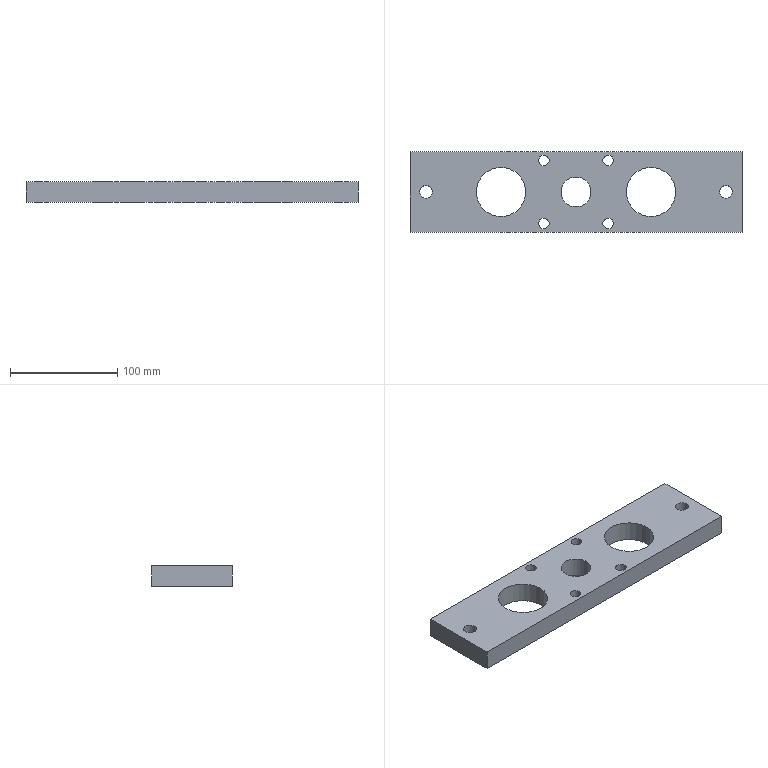Part | NX | features solid 2 | 1 solid | 15 faces | box 310 x 75 x 19 mm | volume 356782 mm3 | cylinder 9 | plane 6 | commonest cylinder face diameters 9.874 x4 12 x2 46 x2 28 x1
STEP:
#1=CARTESIAN_POINT('',(-155.,-117.5,-150.));
#2=VERTEX_POINT('',#1);
#3=CARTESIAN_POINT('',(155.,-117.5,-150.));
#4=VERTEX_POINT('',#3);
#5=CARTESIAN_POINT('',(-155.,-117.5,-150.));
#6=DIRECTION('',(1.,0.,0.));
#7=VECTOR('',#6,1000.);
#8=LINE('',#5,#7);
#9=EDGE_CURVE('',#2,#4,#8,.T.);
#10=ORIENTED_EDGE('',*,*,#9,.F.);
#11=CARTESIAN_POINT('',(-155.,-117.5,-131.));
#12=VERTEX_POINT('',#11);
#13=CARTESIAN_POINT('',(-155.,-117.5,-131.));
#14=DIRECTION('',(0.,0.,-1.));
#15=VECTOR('',#14,1000.);
#16=LINE('',#13,#15);
#17=EDGE_CURVE('',#12,#2,#16,.T.);
#18=ORIENTED_EDGE('',*,*,#17,.F.);
#19=CARTESIAN_POINT('',(155.,-117.5,-131.));
#20=VERTEX_POINT('',#19);
#21=CARTESIAN_POINT('',(-155.,-117.5,-131.));
#22=DIRECTION('',(1.,0.,0.));
#23=VECTOR('',#22,1000.);
#24=LINE('',#21,#23);
#25=EDGE_CURVE('',#12,#20,#24,.T.);
#26=ORIENTED_EDGE('',*,*,#25,.T.);
#27=CARTESIAN_POINT('',(155.,-117.5,-131.));
#28=DIRECTION('',(0.,0.,-1.));
#29=VECTOR('',#28,1000.);
#30=LINE('',#27,#29);
#31=EDGE_CURVE('',#20,#4,#30,.T.);
#32=ORIENTED_EDGE('',*,*,#31,.T.);
#33=EDGE_LOOP('',(#10,#18,#26,#32));
#34=FACE_BOUND('',#33,.T.);
#35=CARTESIAN_POINT('',(-155.,-117.5,-131.));
#36=DIRECTION('',(0.,1.,0.));
#37=DIRECTION('',(0.,0.,1.));
#38=AXIS2_PLACEMENT_3D('',#35,#36,#37);
#39=PLANE('',#38);
#40=ADVANCED_FACE('',(#34),#39,.T.);
#41=CARTESIAN_POINT('',(-155.,-192.5,-150.));
#42=VERTEX_POINT('',#41);
#43=CARTESIAN_POINT('',(-155.,-155.,-150.));
#44=DIRECTION('',(0.,-1.,0.));
#45=VECTOR('',#44,1000.);
#46=LINE('',#43,#45);
#47=EDGE_CURVE('',#2,#42,#46,.T.);
#48=ORIENTED_EDGE('',*,*,#47,.T.);
#49=CARTESIAN_POINT('',(-155.,-192.5,-131.));
#50=VERTEX_POINT('',#49);
#51=CARTESIAN_POINT('',(-155.,-192.5,-131.));
#52=DIRECTION('',(0.,0.,-1.));
#53=VECTOR('',#52,1000.);
#54=LINE('',#51,#53);
#55=EDGE_CURVE('',#50,#42,#54,.T.);
#56=ORIENTED_EDGE('',*,*,#55,.F.);
#57=CARTESIAN_POINT('',(-155.,-155.,-131.));
#58=DIRECTION('',(0.,-1.,0.));
#59=VECTOR('',#58,1000.);
#60=LINE('',#57,#59);
#61=EDGE_CURVE('',#12,#50,#60,.T.);
#62=ORIENTED_EDGE('',*,*,#61,.F.);
#63=ORIENTED_EDGE('',*,*,#17,.T.);
#64=EDGE_LOOP('',(#48,#56,#62,#63));
#65=FACE_BOUND('',#64,.T.);
#66=CARTESIAN_POINT('',(-155.,-155.,-131.));
#67=DIRECTION('',(1.,0.,0.));
#68=DIRECTION('',(0.,0.,-1.));
#69=AXIS2_PLACEMENT_3D('',#66,#67,#68);
#70=PLANE('',#69);
#71=ADVANCED_FACE('',(#65),#70,.F.);
#72=CARTESIAN_POINT('',(155.,-192.5,-150.));
#73=VERTEX_POINT('',#72);
#74=CARTESIAN_POINT('',(155.,-192.5,-150.));
#75=DIRECTION('',(-1.,0.,0.));
#76=VECTOR('',#75,1000.);
#77=LINE('',#74,#76);
#78=EDGE_CURVE('',#73,#42,#77,.T.);
#79=ORIENTED_EDGE('',*,*,#78,.F.);
#80=CARTESIAN_POINT('',(155.,-192.5,-131.));
#81=VERTEX_POINT('',#80);
#82=CARTESIAN_POINT('',(155.,-192.5,-131.));
#83=DIRECTION('',(0.,0.,-1.));
#84=VECTOR('',#83,1000.);
#85=LINE('',#82,#84);
#86=EDGE_CURVE('',#81,#73,#85,.T.);
#87=ORIENTED_EDGE('',*,*,#86,.F.);
#88=CARTESIAN_POINT('',(155.,-192.5,-131.));
#89=DIRECTION('',(-1.,0.,0.));
#90=VECTOR('',#89,1000.);
#91=LINE('',#88,#90);
#92=EDGE_CURVE('',#81,#50,#91,.T.);
#93=ORIENTED_EDGE('',*,*,#92,.T.);
#94=ORIENTED_EDGE('',*,*,#55,.T.);
#95=EDGE_LOOP('',(#79,#87,#93,#94));
#96=FACE_BOUND('',#95,.T.);
#97=CARTESIAN_POINT('',(155.,-192.5,-131.));
#98=DIRECTION('',(0.,-1.,0.));
#99=DIRECTION('',(1.,0.,0.));
#100=AXIS2_PLACEMENT_3D('',#97,#98,#99);
#101=PLANE('',#100);
#102=ADVANCED_FACE('',(#96),#101,.T.);
#103=CARTESIAN_POINT('',(-34.937,-125.594,-131.));
#104=VERTEX_POINT('',#103);
#105=CARTESIAN_POINT('',(-30.,-125.594,-131.));
#106=DIRECTION('',(0.,0.,1.));
#107=DIRECTION('',(-1.,0.,0.));
#108=AXIS2_PLACEMENT_3D('',#105,#106,#107);
#109=CIRCLE('',#108,4.937);
#110=EDGE_CURVE('',#104,#104,#109,.T.);
#111=ORIENTED_EDGE('',*,*,#110,.T.);
#112=EDGE_LOOP('',(#111));
#113=FACE_BOUND('',#112,.T.);
#114=CARTESIAN_POINT('',(-34.937,-125.594,-150.));
#115=VERTEX_POINT('',#114);
#116=CARTESIAN_POINT('',(-30.,-125.594,-150.));
#117=DIRECTION('',(0.,0.,1.));
#118=DIRECTION('',(-1.,0.,0.));
#119=AXIS2_PLACEMENT_3D('',#116,#117,#118);
#120=CIRCLE('',#119,4.937);
#121=EDGE_CURVE('',#115,#115,#120,.T.);
#122=ORIENTED_EDGE('',*,*,#121,.F.);
#123=EDGE_LOOP('',(#122));
#124=FACE_BOUND('',#123,.T.);
#125=CARTESIAN_POINT('',(-30.,-125.594,-131.));
#126=DIRECTION('',(0.,0.,-1.));
#127=DIRECTION('',(-1.,0.,0.));
#128=AXIS2_PLACEMENT_3D('',#125,#126,#127);
#129=CYLINDRICAL_SURFACE('',#128,4.937);
#130=ADVANCED_FACE('',(#113,#124),#129,.F.);
#131=CARTESIAN_POINT('',(47.,-155.,-131.));
#132=VERTEX_POINT('',#131);
#133=CARTESIAN_POINT('',(70.,-155.,-131.));
#134=DIRECTION('',(0.,0.,-1.));
#135=DIRECTION('',(-1.,0.,0.));
#136=AXIS2_PLACEMENT_3D('',#133,#134,#135);
#137=CIRCLE('',#136,23.);
#138=EDGE_CURVE('',#132,#132,#137,.T.);
#139=ORIENTED_EDGE('',*,*,#138,.F.);
#140=EDGE_LOOP('',(#139));
#141=FACE_BOUND('',#140,.T.);
#142=CARTESIAN_POINT('',(47.,-155.,-150.));
#143=VERTEX_POINT('',#142);
#144=CARTESIAN_POINT('',(70.,-155.,-150.));
#145=DIRECTION('',(0.,0.,-1.));
#146=DIRECTION('',(-1.,0.,0.));
#147=AXIS2_PLACEMENT_3D('',#144,#145,#146);
#148=CIRCLE('',#147,23.);
#149=EDGE_CURVE('',#143,#143,#148,.T.);
#150=ORIENTED_EDGE('',*,*,#149,.T.);
#151=EDGE_LOOP('',(#150));
#152=FACE_BOUND('',#151,.T.);
#153=CARTESIAN_POINT('',(70.,-155.,-131.));
#154=DIRECTION('',(0.,0.,-1.));
#155=DIRECTION('',(-1.,0.,0.));
#156=AXIS2_PLACEMENT_3D('',#153,#154,#155);
#157=CYLINDRICAL_SURFACE('',#156,23.);
#158=ADVANCED_FACE('',(#141,#152),#157,.F.);
#159=CARTESIAN_POINT('',(-134.,-155.,-131.));
#160=VERTEX_POINT('',#159);
#161=CARTESIAN_POINT('',(-140.,-155.,-131.));
#162=DIRECTION('',(0.,0.,1.));
#163=DIRECTION('',(1.,0.,0.));
#164=AXIS2_PLACEMENT_3D('',#161,#162,#163);
#165=CIRCLE('',#164,6.);
#166=EDGE_CURVE('',#160,#160,#165,.T.);
#167=ORIENTED_EDGE('',*,*,#166,.T.);
#168=EDGE_LOOP('',(#167));
#169=FACE_BOUND('',#168,.T.);
#170=CARTESIAN_POINT('',(-134.,-155.,-150.));
#171=VERTEX_POINT('',#170);
#172=CARTESIAN_POINT('',(-140.,-155.,-150.));
#173=DIRECTION('',(0.,0.,1.));
#174=DIRECTION('',(1.,0.,0.));
#175=AXIS2_PLACEMENT_3D('',#172,#173,#174);
#176=CIRCLE('',#175,6.);
#177=EDGE_CURVE('',#171,#171,#176,.T.);
#178=ORIENTED_EDGE('',*,*,#177,.F.);
#179=EDGE_LOOP('',(#178));
#180=FACE_BOUND('',#179,.T.);
#181=CARTESIAN_POINT('',(-140.,-155.,-131.));
#182=DIRECTION('',(0.,0.,-1.));
#183=DIRECTION('',(-1.,0.,0.));
#184=AXIS2_PLACEMENT_3D('',#181,#182,#183);
#185=CYLINDRICAL_SURFACE('',#184,6.);
#186=ADVANCED_FACE('',(#169,#180),#185,.F.);
#187=CARTESIAN_POINT('',(155.,-155.,-150.));
#188=DIRECTION('',(0.,-1.,0.));
#189=VECTOR('',#188,1000.);
#190=LINE('',#187,#189);
#191=EDGE_CURVE('',#4,#73,#190,.T.);
#192=ORIENTED_EDGE('',*,*,#191,.F.);
#193=ORIENTED_EDGE('',*,*,#31,.F.);
#194=CARTESIAN_POINT('',(155.,-155.,-131.));
#195=DIRECTION('',(0.,-1.,0.));
#196=VECTOR('',#195,1000.);
#197=LINE('',#194,#196);
#198=EDGE_CURVE('',#20,#81,#197,.T.);
#199=ORIENTED_EDGE('',*,*,#198,.T.);
#200=ORIENTED_EDGE('',*,*,#86,.T.);
#201=EDGE_LOOP('',(#192,#193,#199,#200));
#202=FACE_BOUND('',#201,.T.);
#203=CARTESIAN_POINT('',(155.,-155.,-131.));
#204=DIRECTION('',(1.,0.,0.));
#205=DIRECTION('',(0.,0.,-1.));
#206=AXIS2_PLACEMENT_3D('',#203,#204,#205);
#207=PLANE('',#206);
#208=ADVANCED_FACE('',(#202),#207,.T.);
#209=CARTESIAN_POINT('',(134.,-155.,-131.));
#210=VERTEX_POINT('',#209);
#211=CARTESIAN_POINT('',(140.,-155.,-131.));
#212=DIRECTION('',(0.,0.,-1.));
#213=DIRECTION('',(-1.,0.,0.));
#214=AXIS2_PLACEMENT_3D('',#211,#212,#213);
#215=CIRCLE('',#214,6.);
#216=EDGE_CURVE('',#210,#210,#215,.T.);
#217=ORIENTED_EDGE('',*,*,#216,.F.);
#218=EDGE_LOOP('',(#217));
#219=FACE_BOUND('',#218,.T.);
#220=CARTESIAN_POINT('',(134.,-155.,-150.));
#221=VERTEX_POINT('',#220);
#222=CARTESIAN_POINT('',(140.,-155.,-150.));
#223=DIRECTION('',(0.,0.,-1.));
#224=DIRECTION('',(-1.,0.,0.));
#225=AXIS2_PLACEMENT_3D('',#222,#223,#224);
#226=CIRCLE('',#225,6.);
#227=EDGE_CURVE('',#221,#221,#226,.T.);
#228=ORIENTED_EDGE('',*,*,#227,.T.);
#229=EDGE_LOOP('',(#228));
#230=FACE_BOUND('',#229,.T.);
#231=CARTESIAN_POINT('',(140.,-155.,-131.));
#232=DIRECTION('',(0.,0.,-1.));
#233=DIRECTION('',(-1.,0.,0.));
#234=AXIS2_PLACEMENT_3D('',#231,#232,#233);
#235=CYLINDRICAL_SURFACE('',#234,6.);
#236=ADVANCED_FACE('',(#219,#230),#235,.F.);
#237=CARTESIAN_POINT('',(-47.,-155.,-131.));
#238=VERTEX_POINT('',#237);
#239=CARTESIAN_POINT('',(-70.,-155.,-131.));
#240=DIRECTION('',(0.,0.,1.));
#241=DIRECTION('',(1.,0.,0.));
#242=AXIS2_PLACEMENT_3D('',#239,#240,#241);
#243=CIRCLE('',#242,23.);
#244=EDGE_CURVE('',#238,#238,#243,.T.);
#245=ORIENTED_EDGE('',*,*,#244,.T.);
#246=EDGE_LOOP('',(#245));
#247=FACE_BOUND('',#246,.T.);
#248=CARTESIAN_POINT('',(-47.,-155.,-150.));
#249=VERTEX_POINT('',#248);
#250=CARTESIAN_POINT('',(-70.,-155.,-150.));
#251=DIRECTION('',(0.,0.,1.));
#252=DIRECTION('',(1.,0.,0.));
#253=AXIS2_PLACEMENT_3D('',#250,#251,#252);
#254=CIRCLE('',#253,23.);
#255=EDGE_CURVE('',#249,#249,#254,.T.);
#256=ORIENTED_EDGE('',*,*,#255,.F.);
#257=EDGE_LOOP('',(#256));
#258=FACE_BOUND('',#257,.T.);
#259=CARTESIAN_POINT('',(-70.,-155.,-131.));
#260=DIRECTION('',(0.,0.,-1.));
#261=DIRECTION('',(-1.,0.,0.));
#262=AXIS2_PLACEMENT_3D('',#259,#260,#261);
#263=CYLINDRICAL_SURFACE('',#262,23.);
#264=ADVANCED_FACE('',(#247,#258),#263,.F.);
#265=CARTESIAN_POINT('',(34.937,-125.594,-131.));
#266=VERTEX_POINT('',#265);
#267=CARTESIAN_POINT('',(30.,-125.594,-131.));
#268=DIRECTION('',(0.,0.,-1.));
#269=DIRECTION('',(1.,0.,0.));
#270=AXIS2_PLACEMENT_3D('',#267,#268,#269);
#271=CIRCLE('',#270,4.937);
#272=EDGE_CURVE('',#266,#266,#271,.T.);
#273=ORIENTED_EDGE('',*,*,#272,.F.);
#274=EDGE_LOOP('',(#273));
#275=FACE_BOUND('',#274,.T.);
#276=CARTESIAN_POINT('',(34.937,-125.594,-150.));
#277=VERTEX_POINT('',#276);
#278=CARTESIAN_POINT('',(30.,-125.594,-150.));
#279=DIRECTION('',(0.,0.,-1.));
#280=DIRECTION('',(1.,0.,0.));
#281=AXIS2_PLACEMENT_3D('',#278,#279,#280);
#282=CIRCLE('',#281,4.937);
#283=EDGE_CURVE('',#277,#277,#282,.T.);
#284=ORIENTED_EDGE('',*,*,#283,.T.);
#285=EDGE_LOOP('',(#284));
#286=FACE_BOUND('',#285,.T.);
#287=CARTESIAN_POINT('',(30.,-125.594,-131.));
#288=DIRECTION('',(0.,0.,-1.));
#289=DIRECTION('',(-1.,0.,0.));
#290=AXIS2_PLACEMENT_3D('',#287,#288,#289);
#291=CYLINDRICAL_SURFACE('',#290,4.937);
#292=ADVANCED_FACE('',(#275,#286),#291,.F.);
#293=CARTESIAN_POINT('',(34.937,-184.406,-131.));
#294=VERTEX_POINT('',#293);
#295=CARTESIAN_POINT('',(30.,-184.406,-131.));
#296=DIRECTION('',(0.,0.,1.));
#297=DIRECTION('',(1.,0.,0.));
#298=AXIS2_PLACEMENT_3D('',#295,#296,#297);
#299=CIRCLE('',#298,4.937);
#300=EDGE_CURVE('',#294,#294,#299,.T.);
#301=ORIENTED_EDGE('',*,*,#300,.T.);
#302=EDGE_LOOP('',(#301));
#303=FACE_BOUND('',#302,.T.);
#304=CARTESIAN_POINT('',(34.937,-184.406,-150.));
#305=VERTEX_POINT('',#304);
#306=CARTESIAN_POINT('',(30.,-184.406,-150.));
#307=DIRECTION('',(0.,0.,1.));
#308=DIRECTION('',(1.,0.,0.));
#309=AXIS2_PLACEMENT_3D('',#306,#307,#308);
#310=CIRCLE('',#309,4.937);
#311=EDGE_CURVE('',#305,#305,#310,.T.);
#312=ORIENTED_EDGE('',*,*,#311,.F.);
#313=EDGE_LOOP('',(#312));
#314=FACE_BOUND('',#313,.T.);
#315=CARTESIAN_POINT('',(30.,-184.406,-131.));
#316=DIRECTION('',(0.,0.,-1.));
#317=DIRECTION('',(-1.,0.,0.));
#318=AXIS2_PLACEMENT_3D('',#315,#316,#317);
#319=CYLINDRICAL_SURFACE('',#318,4.937);
#320=ADVANCED_FACE('',(#303,#314),#319,.F.);
#321=CARTESIAN_POINT('',(14.,-155.,-131.));
#322=VERTEX_POINT('',#321);
#323=CARTESIAN_POINT('',(0.,-155.,-131.));
#324=DIRECTION('',(0.,0.,1.));
#325=DIRECTION('',(1.,0.,0.));
#326=AXIS2_PLACEMENT_3D('',#323,#324,#325);
#327=CIRCLE('',#326,14.);
#328=EDGE_CURVE('',#322,#322,#327,.T.);
#329=ORIENTED_EDGE('',*,*,#328,.T.);
#330=EDGE_LOOP('',(#329));
#331=FACE_BOUND('',#330,.T.);
#332=CARTESIAN_POINT('',(14.,-155.,-150.));
#333=VERTEX_POINT('',#332);
#334=CARTESIAN_POINT('',(0.,-155.,-150.));
#335=DIRECTION('',(0.,0.,1.));
#336=DIRECTION('',(1.,0.,0.));
#337=AXIS2_PLACEMENT_3D('',#334,#335,#336);
#338=CIRCLE('',#337,14.);
#339=EDGE_CURVE('',#333,#333,#338,.T.);
#340=ORIENTED_EDGE('',*,*,#339,.F.);
#341=EDGE_LOOP('',(#340));
#342=FACE_BOUND('',#341,.T.);
#343=CARTESIAN_POINT('',(0.,-155.,-131.));
#344=DIRECTION('',(0.,0.,-1.));
#345=DIRECTION('',(-1.,0.,0.));
#346=AXIS2_PLACEMENT_3D('',#343,#344,#345);
#347=CYLINDRICAL_SURFACE('',#346,14.);
#348=ADVANCED_FACE('',(#331,#342),#347,.F.);
#349=CARTESIAN_POINT('',(-34.937,-184.406,-131.));
#350=VERTEX_POINT('',#349);
#351=CARTESIAN_POINT('',(-30.,-184.406,-131.));
#352=DIRECTION('',(0.,0.,-1.));
#353=DIRECTION('',(-1.,0.,0.));
#354=AXIS2_PLACEMENT_3D('',#351,#352,#353);
#355=CIRCLE('',#354,4.937);
#356=EDGE_CURVE('',#350,#350,#355,.T.);
#357=ORIENTED_EDGE('',*,*,#356,.F.);
#358=EDGE_LOOP('',(#357));
#359=FACE_BOUND('',#358,.T.);
#360=CARTESIAN_POINT('',(-34.937,-184.406,-150.));
#361=VERTEX_POINT('',#360);
#362=CARTESIAN_POINT('',(-30.,-184.406,-150.));
#363=DIRECTION('',(0.,0.,-1.));
#364=DIRECTION('',(-1.,0.,0.));
#365=AXIS2_PLACEMENT_3D('',#362,#363,#364);
#366=CIRCLE('',#365,4.937);
#367=EDGE_CURVE('',#361,#361,#366,.T.);
#368=ORIENTED_EDGE('',*,*,#367,.T.);
#369=EDGE_LOOP('',(#368));
#370=FACE_BOUND('',#369,.T.);
#371=CARTESIAN_POINT('',(-30.,-184.406,-131.));
#372=DIRECTION('',(0.,0.,-1.));
#373=DIRECTION('',(-1.,0.,0.));
#374=AXIS2_PLACEMENT_3D('',#371,#372,#373);
#375=CYLINDRICAL_SURFACE('',#374,4.937);
#376=ADVANCED_FACE('',(#359,#370),#375,.F.);
#377=ORIENTED_EDGE('',*,*,#328,.F.);
#378=EDGE_LOOP('',(#377));
#379=FACE_BOUND('',#378,.T.);
#380=ORIENTED_EDGE('',*,*,#300,.F.);
#381=EDGE_LOOP('',(#380));
#382=FACE_BOUND('',#381,.T.);
#383=ORIENTED_EDGE('',*,*,#272,.T.);
#384=EDGE_LOOP('',(#383));
#385=FACE_BOUND('',#384,.T.);
#386=ORIENTED_EDGE('',*,*,#244,.F.);
#387=EDGE_LOOP('',(#386));
#388=FACE_BOUND('',#387,.T.);
#389=ORIENTED_EDGE('',*,*,#216,.T.);
#390=EDGE_LOOP('',(#389));
#391=FACE_BOUND('',#390,.T.);
#392=ORIENTED_EDGE('',*,*,#198,.F.);
#393=ORIENTED_EDGE('',*,*,#25,.F.);
#394=ORIENTED_EDGE('',*,*,#61,.T.);
#395=ORIENTED_EDGE('',*,*,#92,.F.);
#396=EDGE_LOOP('',(#392,#393,#394,#395));
#397=FACE_BOUND('',#396,.T.);
#398=ORIENTED_EDGE('',*,*,#166,.F.);
#399=EDGE_LOOP('',(#398));
#400=FACE_BOUND('',#399,.T.);
#401=ORIENTED_EDGE('',*,*,#138,.T.);
#402=EDGE_LOOP('',(#401));
#403=FACE_BOUND('',#402,.T.);
#404=ORIENTED_EDGE('',*,*,#110,.F.);
#405=EDGE_LOOP('',(#404));
#406=FACE_BOUND('',#405,.T.);
#407=ORIENTED_EDGE('',*,*,#356,.T.);
#408=EDGE_LOOP('',(#407));
#409=FACE_BOUND('',#408,.T.);
#410=CARTESIAN_POINT('',(155.,-192.5,-131.));
#411=DIRECTION('',(0.,0.,-1.));
#412=DIRECTION('',(-1.,0.,0.));
#413=AXIS2_PLACEMENT_3D('',#410,#411,#412);
#414=PLANE('',#413);
#415=ADVANCED_FACE('',(#379,#382,#385,#388,#391,#397,#400,#403,#406,#409),#414,.F.);
#416=ORIENTED_EDGE('',*,*,#339,.T.);
#417=EDGE_LOOP('',(#416));
#418=FACE_BOUND('',#417,.T.);
#419=ORIENTED_EDGE('',*,*,#311,.T.);
#420=EDGE_LOOP('',(#419));
#421=FACE_BOUND('',#420,.T.);
#422=ORIENTED_EDGE('',*,*,#283,.F.);
#423=EDGE_LOOP('',(#422));
#424=FACE_BOUND('',#423,.T.);
#425=ORIENTED_EDGE('',*,*,#255,.T.);
#426=EDGE_LOOP('',(#425));
#427=FACE_BOUND('',#426,.T.);
#428=ORIENTED_EDGE('',*,*,#227,.F.);
#429=EDGE_LOOP('',(#428));
#430=FACE_BOUND('',#429,.T.);
#431=ORIENTED_EDGE('',*,*,#9,.T.);
#432=ORIENTED_EDGE('',*,*,#191,.T.);
#433=ORIENTED_EDGE('',*,*,#78,.T.);
#434=ORIENTED_EDGE('',*,*,#47,.F.);
#435=EDGE_LOOP('',(#431,#432,#433,#434));
#436=FACE_BOUND('',#435,.T.);
#437=ORIENTED_EDGE('',*,*,#177,.T.);
#438=EDGE_LOOP('',(#437));
#439=FACE_BOUND('',#438,.T.);
#440=ORIENTED_EDGE('',*,*,#149,.F.);
#441=EDGE_LOOP('',(#440));
#442=FACE_BOUND('',#441,.T.);
#443=ORIENTED_EDGE('',*,*,#121,.T.);
#444=EDGE_LOOP('',(#443));
#445=FACE_BOUND('',#444,.T.);
#446=ORIENTED_EDGE('',*,*,#367,.F.);
#447=EDGE_LOOP('',(#446));
#448=FACE_BOUND('',#447,.T.);
#449=CARTESIAN_POINT('',(155.,-192.5,-150.));
#450=DIRECTION('',(0.,0.,-1.));
#451=DIRECTION('',(-1.,0.,0.));
#452=AXIS2_PLACEMENT_3D('',#449,#450,#451);
#453=PLANE('',#452);
#454=ADVANCED_FACE('',(#418,#421,#424,#427,#430,#436,#439,#442,#445,#448),#453,.T.);
#455=CLOSED_SHELL('',(#40,#71,#102,#130,#158,#186,#208,#236,#264,#292,#320,#348,#376,#415,#454));
#456=MANIFOLD_SOLID_BREP('',#455);
#457=(LENGTH_UNIT()NAMED_UNIT(*)SI_UNIT(.MILLI.,.METRE.));
#458=UNCERTAINTY_MEASURE_WITH_UNIT(LENGTH_MEASURE(0.00001),#457,'','');
#459=(NAMED_UNIT(*)PLANE_ANGLE_UNIT()SI_UNIT($,.RADIAN.));
#460=(NAMED_UNIT(*)SI_UNIT($,.STERADIAN.)SOLID_ANGLE_UNIT());
#461=(GEOMETRIC_REPRESENTATION_CONTEXT(3)GLOBAL_UNCERTAINTY_ASSIGNED_CONTEXT((#458))GLOBAL_UNIT_ASSIGNED_CONTEXT((#457,#459,#460))REPRESENTATION_CONTEXT('',''));
#462=ADVANCED_BREP_SHAPE_REPRESENTATION('',(#456),#461);